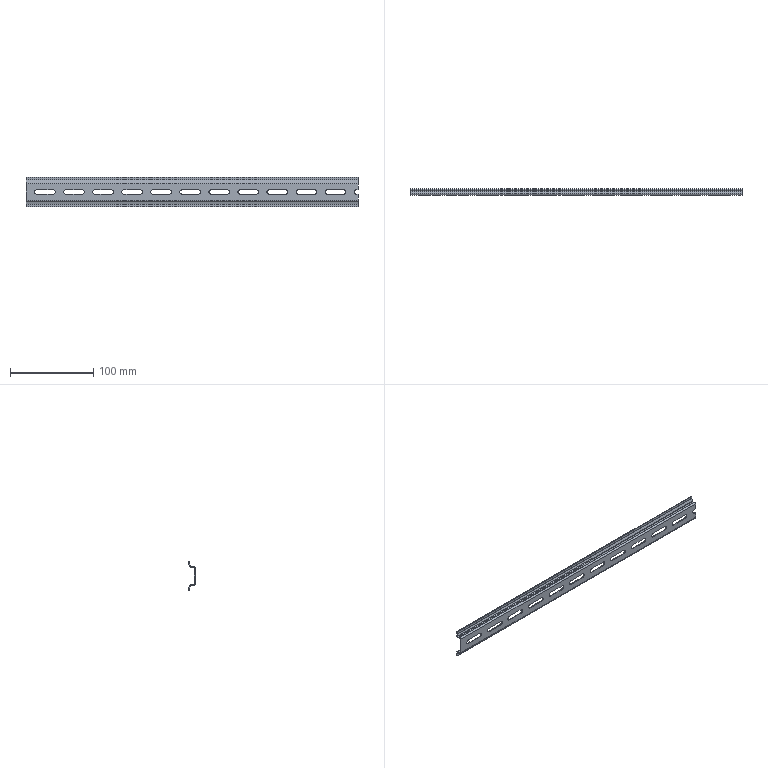Part | SolidWorks | features BaseBody 1 | 1 solid | 82 faces | box 400 x 7.5 x 35.04 mm | volume 16816 mm3 | plane 43 | cylinder 39 | commonest cylinder face diameters 5.352 x23 1.473 x8 3.473 x8